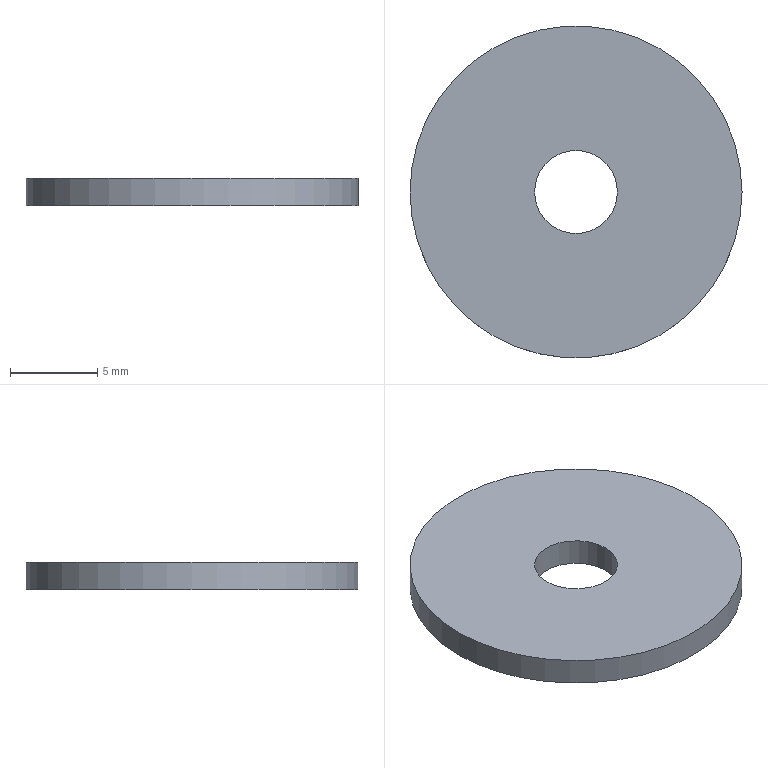Part | NX | features door hinge 2(left) 2 | 1 solid | 4 faces | box 19.05 x 19.05 x 1.575 mm | volume 420.801 mm3 | cylinder 2 | plane 2 | commonest cylinder face diameters 4.763 x1 19.05 x1
STEP:
#1=CARTESIAN_POINT('',(-7.165,-18.613,3.162));
#2=VERTEX_POINT('',#1);
#3=CARTESIAN_POINT('',(-16.69,-18.613,3.162));
#4=DIRECTION('',(0.,0.,1.));
#5=DIRECTION('',(1.,0.,0.));
#6=AXIS2_PLACEMENT_3D('',#3,#4,#5);
#7=CIRCLE('',#6,9.525);
#8=EDGE_CURVE('',#2,#2,#7,.T.);
#9=ORIENTED_EDGE('',*,*,#8,.F.);
#10=EDGE_LOOP('',(#9));
#11=FACE_BOUND('',#10,.T.);
#12=CARTESIAN_POINT('',(-7.165,-18.613,1.587));
#13=VERTEX_POINT('',#12);
#14=CARTESIAN_POINT('',(-16.69,-18.613,1.587));
#15=DIRECTION('',(0.,0.,1.));
#16=DIRECTION('',(1.,0.,0.));
#17=AXIS2_PLACEMENT_3D('',#14,#15,#16);
#18=CIRCLE('',#17,9.525);
#19=EDGE_CURVE('',#13,#13,#18,.T.);
#20=ORIENTED_EDGE('',*,*,#19,.T.);
#21=EDGE_LOOP('',(#20));
#22=FACE_BOUND('',#21,.T.);
#23=CARTESIAN_POINT('',(-16.69,-18.613,3.162));
#24=DIRECTION('',(0.,0.,-1.));
#25=DIRECTION('',(1.,0.,0.));
#26=AXIS2_PLACEMENT_3D('',#23,#24,#25);
#27=CYLINDRICAL_SURFACE('',#26,9.525);
#28=ADVANCED_FACE('',(#11,#22),#27,.T.);
#29=CARTESIAN_POINT('',(-14.309,-18.613,3.162));
#30=VERTEX_POINT('',#29);
#31=CARTESIAN_POINT('',(-16.69,-18.613,3.162));
#32=DIRECTION('',(0.,0.,1.));
#33=DIRECTION('',(1.,0.,0.));
#34=AXIS2_PLACEMENT_3D('',#31,#32,#33);
#35=CIRCLE('',#34,2.381);
#36=EDGE_CURVE('',#30,#30,#35,.T.);
#37=ORIENTED_EDGE('',*,*,#36,.F.);
#38=EDGE_LOOP('',(#37));
#39=FACE_BOUND('',#38,.T.);
#40=ORIENTED_EDGE('',*,*,#8,.T.);
#41=EDGE_LOOP('',(#40));
#42=FACE_BOUND('',#41,.T.);
#43=CARTESIAN_POINT('',(-16.69,-18.613,3.162));
#44=DIRECTION('',(0.,0.,-1.));
#45=DIRECTION('',(1.,0.,0.));
#46=AXIS2_PLACEMENT_3D('',#43,#44,#45);
#47=PLANE('',#46);
#48=ADVANCED_FACE('',(#39,#42),#47,.F.);
#49=CARTESIAN_POINT('',(-14.309,-18.613,1.587));
#50=VERTEX_POINT('',#49);
#51=CARTESIAN_POINT('',(-16.69,-18.613,1.587));
#52=DIRECTION('',(0.,0.,1.));
#53=DIRECTION('',(1.,0.,0.));
#54=AXIS2_PLACEMENT_3D('',#51,#52,#53);
#55=CIRCLE('',#54,2.381);
#56=EDGE_CURVE('',#50,#50,#55,.T.);
#57=ORIENTED_EDGE('',*,*,#56,.T.);
#58=EDGE_LOOP('',(#57));
#59=FACE_BOUND('',#58,.T.);
#60=ORIENTED_EDGE('',*,*,#19,.F.);
#61=EDGE_LOOP('',(#60));
#62=FACE_BOUND('',#61,.T.);
#63=CARTESIAN_POINT('',(-16.69,-18.613,1.587));
#64=DIRECTION('',(0.,0.,-1.));
#65=DIRECTION('',(1.,0.,0.));
#66=AXIS2_PLACEMENT_3D('',#63,#64,#65);
#67=PLANE('',#66);
#68=ADVANCED_FACE('',(#59,#62),#67,.T.);
#69=ORIENTED_EDGE('',*,*,#36,.T.);
#70=EDGE_LOOP('',(#69));
#71=FACE_BOUND('',#70,.T.);
#72=ORIENTED_EDGE('',*,*,#56,.F.);
#73=EDGE_LOOP('',(#72));
#74=FACE_BOUND('',#73,.T.);
#75=CARTESIAN_POINT('',(-16.69,-18.613,3.162));
#76=DIRECTION('',(0.,0.,-1.));
#77=DIRECTION('',(1.,0.,0.));
#78=AXIS2_PLACEMENT_3D('',#75,#76,#77);
#79=CYLINDRICAL_SURFACE('',#78,2.381);
#80=ADVANCED_FACE('',(#71,#74),#79,.F.);
#81=CLOSED_SHELL('',(#28,#48,#68,#80));
#82=MANIFOLD_SOLID_BREP('',#81);
#83=(LENGTH_UNIT()NAMED_UNIT(*)SI_UNIT(.MILLI.,.METRE.));
#84=UNCERTAINTY_MEASURE_WITH_UNIT(LENGTH_MEASURE(0.00001),#83,'','');
#85=(NAMED_UNIT(*)PLANE_ANGLE_UNIT()SI_UNIT($,.RADIAN.));
#86=(NAMED_UNIT(*)SI_UNIT($,.STERADIAN.)SOLID_ANGLE_UNIT());
#87=(GEOMETRIC_REPRESENTATION_CONTEXT(3)GLOBAL_UNCERTAINTY_ASSIGNED_CONTEXT((#84))GLOBAL_UNIT_ASSIGNED_CONTEXT((#83,#85,#86))REPRESENTATION_CONTEXT('',''));
#88=ADVANCED_BREP_SHAPE_REPRESENTATION('',(#82),#87);